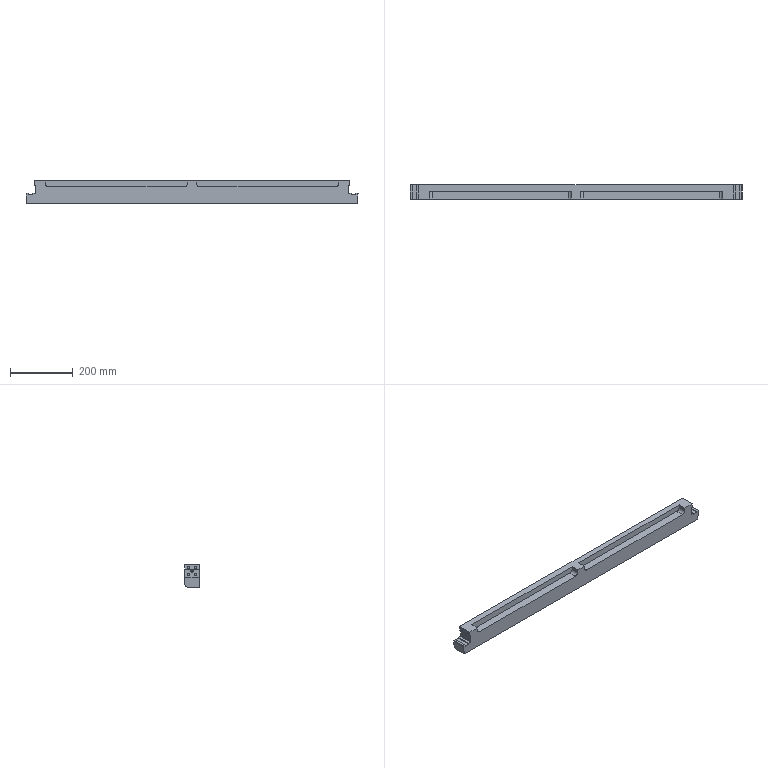Part | 1 solid | 129 faces | box 1056 x 45 x 72.5 mm | volume 2442715 mm3 | plane 60 | cylinder 47 | cone 22 | commonest cylinder face diameters 6.7 x16 6.8 x16 21 x6 20 x5 8 x4